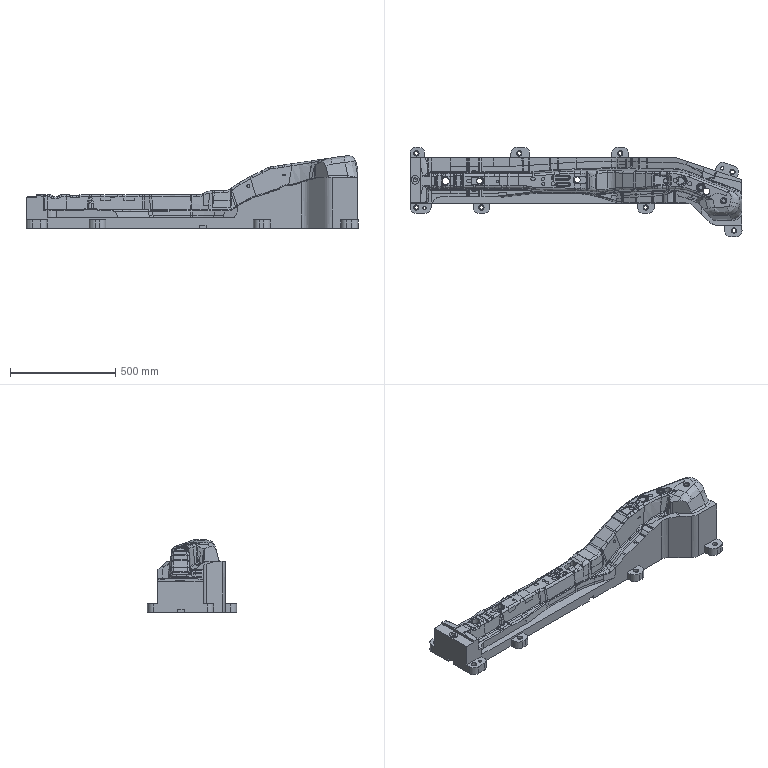Part | NX | features solid 2 | 1 solid | 977 faces | box 1580 x 425 x 345.66 mm | volume 47283863 mm3 | spline 700 | plane 215 | cylinder 59 | cone 2 | sphere 1 | commonest cylinder face diameters 60 x16 20 x10 17.5 x8 25.5 x8 100 x4 16 x2